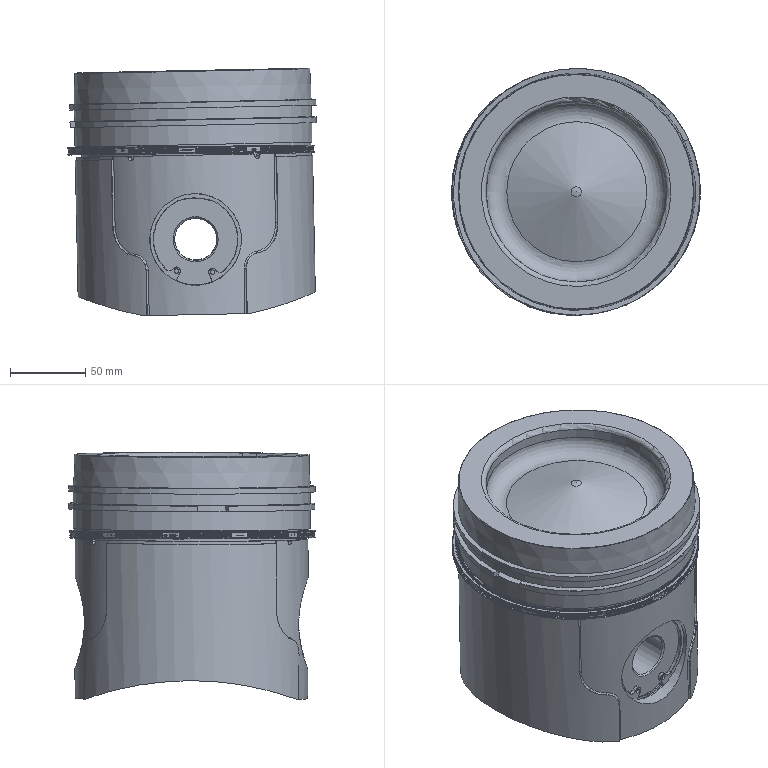Part | NX | features EXTRACT_STRING 371, Instance Feature 369, SWP104 365, EXTRACT_DATUM_AXIS 360, EXTRUDE 27, BLEND 26, DATUM_CSYS 26, SKETCH 20, HOLE PACKAGE 4, TAPER_HOLE 4, MIRROR_SET 3, CHAMFER 2, Pattern Feature 2, CPROJ 1, DATUM_PLANE 1, TEXT 1 | 368 solids | 1752 faces | box 165.688 x 164.309 x 164.424 mm | volume 1799069 mm3 | plane 825 | torus 757 | cylinder 104 | spline 48 | cone 16 | sphere 2 | commonest cylinder face diameters 2 x16 0.4 x8 10 x8 40 x6 61 x5 3 x4